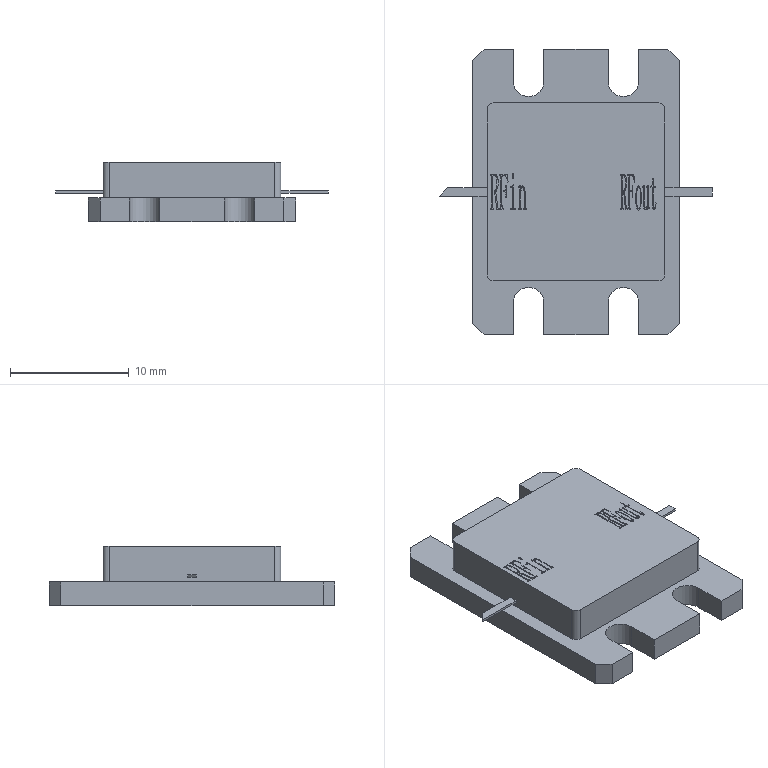Part | STEP file | GN5359P300V40 | 1 solid | 220 faces | box 23 x 24.1 x 5 mm | volume 1437 mm3 | plane 120 | other 92 | cylinder 8 | commonest cylinder face diameters 1 x4 2.6 x4